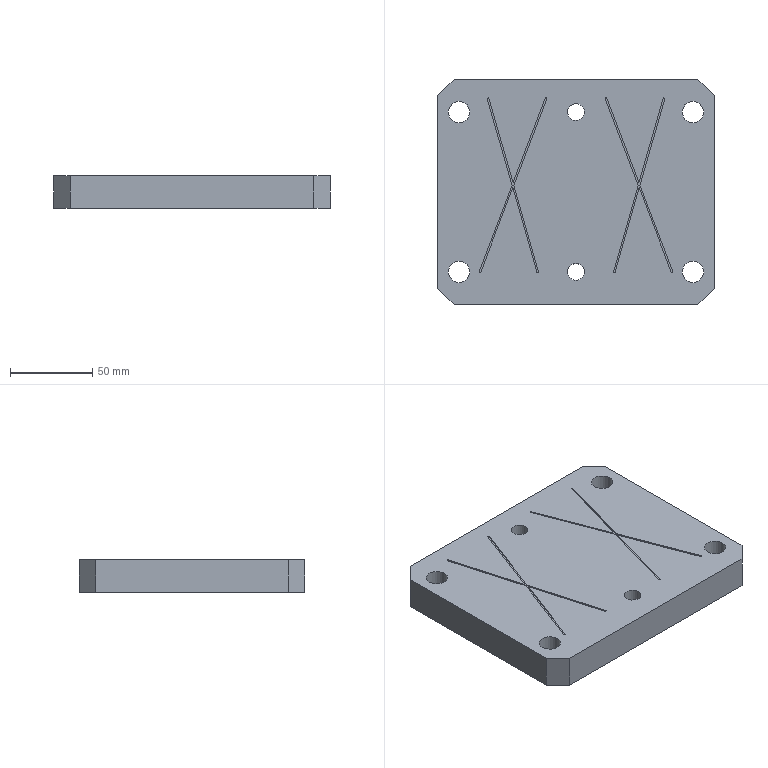Part | STEP file | 1_id622_x_t | 1 solid | 42 faces | box 168 x 137 x 20 mm | volume 442179 mm3 | plane 28 | cylinder 14 | commonest cylinder face diameters 1 x8 13 x4 10.25 x2